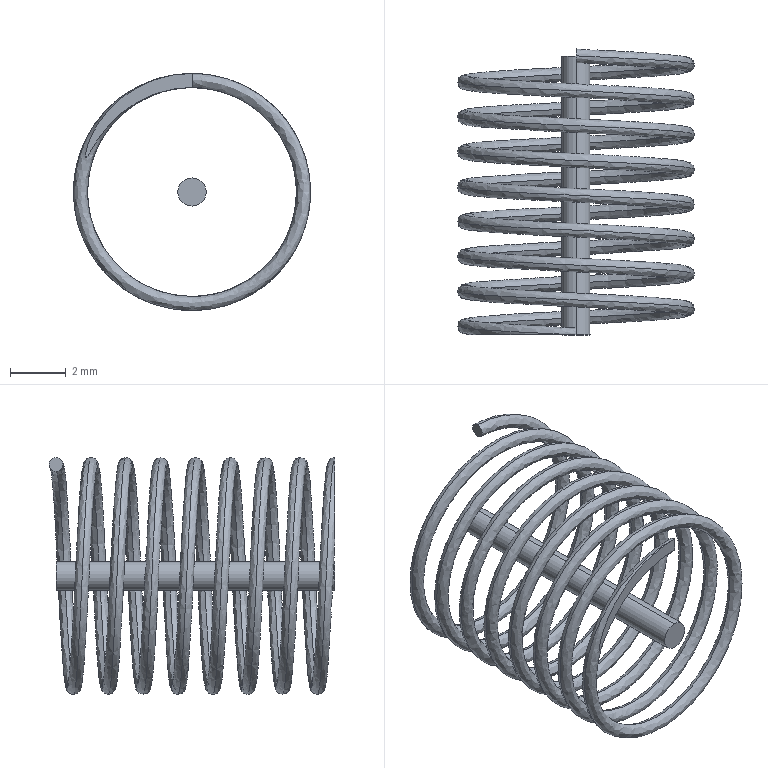Part | SolidWorks | features ICE 2, Helix 1, Sweep 1 | 2 solids | 9 faces | box 8.5 x 10.25 x 8.5 mm | volume 47.392 mm3 | plane 5 | spline 2 | cylinder 2 | commonest cylinder face diameters 1.013 x2